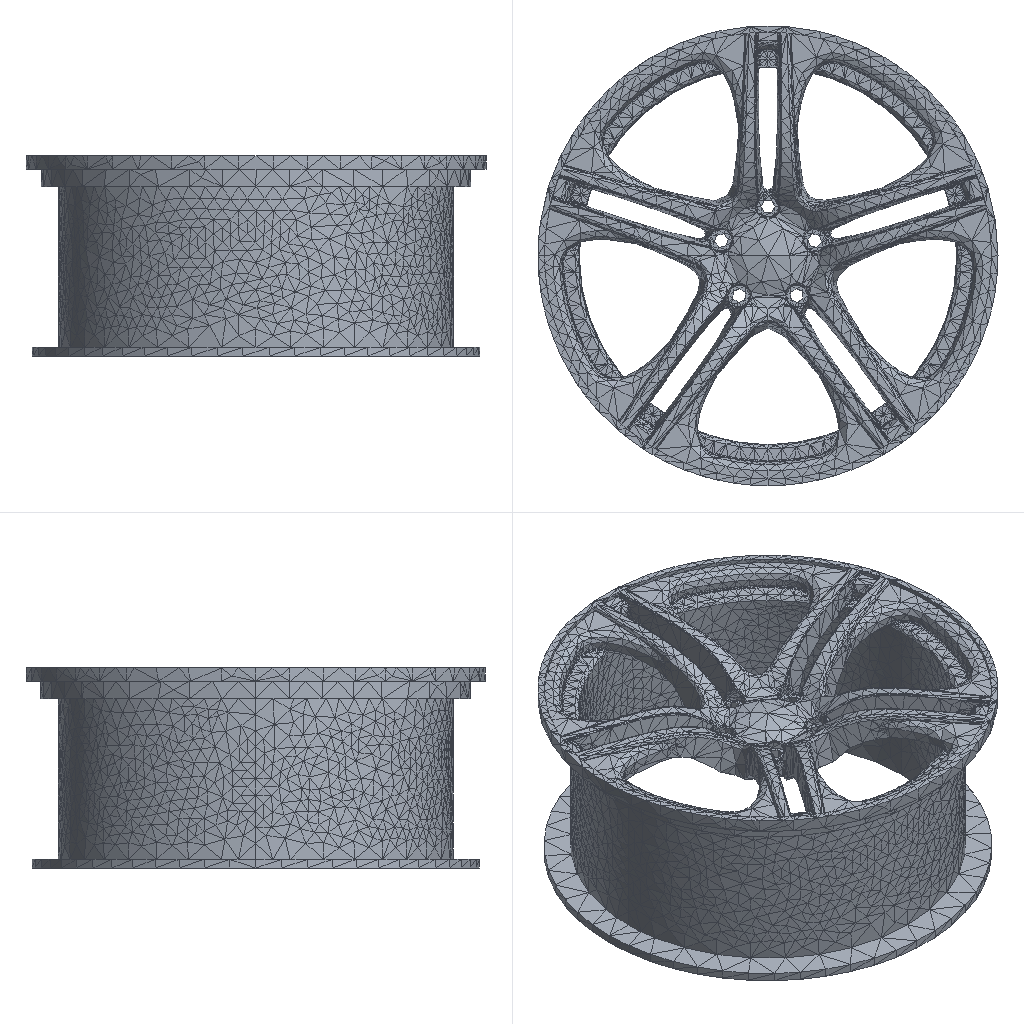Simulation study | ansys workbench
Set-up summary:
category,name,step,type,value,unit,region
solver,ansys_workbench
units,mm-N-s-tonne (MPa),,stated,"/units,MPA"
analysis,LS1,,static
load_step,LS1,LS1,static,nsubst=1; time=1
mesh,nodes,,,48207
mesh,elements,,,28205
element_type,SOLID187,,,25767
element_type,SURF154,,,2438
material,Structural Steel,,E,200000,tonne s^-2 mm^-1
material,Structural Steel,,nu,0.3
material,Structural Steel,,density,7.85e-09,tonne mm^-3
material,Structural Steel,,conductivity,60.5,tonne mm s^-3 C^-1
material,Structural Steel,,specific_heat,4.34e+08,mm^2 s^-2 C^-1
material,Structural Steel,,cte,1.2e-05,C^-1
material,Structural Steel,,permeability,10000
material,Structural Steel,,resistivity,0.00017,ohm mm
load,Define Force Using Surface Effect Elements,LS1,surface-effect pres face 2,-0.01932,,SURF154 #2
bc,Fixed Supports,model,fixed,[dofs=ALL],,_FIXEDSU
named_set,______,,node,549
named_set,_FIXEDSU,,node,549
Ansys APDL input file, long lists of numbers shortened:
/batch
/config,noeldb,1     ! force off writing results to database
*get,_wallstrt,active,,time,wall
! ANSYS input file written by Workbench version 2022 R1
! File used for geometry attach:
/title,wbnew--____ (B5)
! ****** Begin Custom Load Command Snippet ******
/COM, ACT Extensions:
/COM,     LSDYNA, 2021.1
/COM,
! ****** End   Custom Load Command Snippet ******
*DIM,_wb_ProjectScratch_dir,string,248
_wb_ProjectScratch_dir(1) = ''
*DIM,_wb_SolverFiles_dir,string,248
_wb_SolverFiles_dir(1) = ''
*DIM,_wb_userfiles_dir,string,248
_wb_userfiles_dir(1) = ''
/com,--- Data in consistent NMM units. See Solving Units in the help system for more information.
/units,MPA
/nopr
/wb,file,start              !  signify a WB generated input file
/prep7
! Turn off shape checking because checks already performed inside WB mesher.
! See help system for more information.
SHPP,OFF,,NOWARN
/nolist
etcon,set             ! allow ANSYS to choose best KEYOP's for 180x elements, resets any applicable keyopt to MAPDL defaults
/com,*********** Nodes for the whole assembly ***********
nblock,3,,53027
(1i9,3e20.9e3)
        1     8.307477225E+01    -1.054488018E+01     8.547377848E+01
! (48206 more lines like these left out)
-1
/wb,elem,start            !  set before creation of elements
/com,*********** Elements for Body 1 "____-FreeParts|RIM[1]" ***********
et,1,187
eblock,19,solid,,25767
(19i9)
        1        1        1        1        0        0        0        0       10        0        1     1683     3030     1743     7730    21022    21875    21021    21039
! (51533 more lines like these left out)
-1
/wb,elem,end               !  done creating elements
/com,*********** Send User Defined Coordinate System(s) ***********
csys,0
toffst,273.15,  ! Temperature offset from absolute zero
/com,*********** Set Reference Temperature ***********
tref,22.
/wb,mat,start              !  starting to send materials
/com,*********** Send Materials ***********
Temperature = 'TEMP' ! Temperature
MP,DENS,1,7.85e-09,	! tonne mm^-3
MP,ALPX,1,1.2e-05,	! C^-1
MP,C,1,434000000,	! mm^2 s^-2 C^-1
MP,KXX,1,60.5,	! tonne mm s^-3 C^-1
MP,RSVX,1,0.00017,	! ohm mm
MP,EX,1,200000,	! tonne s^-2 mm^-1
MP,NUXY,1,0.3,
MP,MURX,1,10000,
/wb,mat,end                !  done sending materials
!************************* Model Summary ********************
!____-FreeParts|RIM[1],	结构钢,	matid,	1
!************************* End Model Summary ********************
! get the diagonal of the bounding box. Needed later for other things
*get,_xmin,node,,mnloc,x
*get,_ymin,node,,mnloc,y
*get,_zmin,node,,mnloc,z
*get,_xmax,node,,mxloc,x
*get,_ymax,node,,mxloc,y
*get,_zmax,node,,mxloc,z
_ASMDIAG=(_xmax-_xmin)*(_xmax-_xmin)+(_ymax-_ymin)*(_ymax-_ymin)+(_zmax-_zmin)*(_zmax-_zmin)
_ASMDIAG=SQRT(_ASMDIAG)
/wb,contact,start          !  starting to send contact
/wb,contact,end            !  done creating contacts
/com,*********** Send Named Selection as Node Component ***********
CMBLOCK,______  ,NODE,      549
(8i10)
        90        91        92        93       151       152       163       164
! (68 more lines like these left out)
/golist
/wb,load,start             !  starting to send loads
/com,*********** Fixed Supports ***********
CMBLOCK,_FIXEDSU,NODE,      549
(8i10)
        90        91        92        93       151       152       163       164
! (68 more lines like these left out)
cmsel,s,_FIXEDSU
d,all,all
nsel,all
/com,*********** Define Force Using Surface Effect Elements ***********
local,12,0,0.,0.,0.,0.,0.,0.
csys,0
et,2,154
eblock,10,,,2438
(15i9)
    39136        2        2        2       12     1969       74     5447     5447     8846     8850     5447    23519
! (2437 more lines like these left out)
-1
esel,s,type,,2
keyop,2,2,1                ! Apply load in local coordinate system
keyop,2,7,1                ! Use original area so load is constant in large deformation
esel,all
/gst,on,on
fini
*get,_numnode,node,0,count
*get,_numelem,elem,0,count
*get, _MAXELEMNUM, elem, 0, NUM, MAX
*get, _MAXNODENUM, node, 0, NUM, MAX
*get, _MAXELEMTYPE, etyp, 0, NUM, MAX
*get, _MAXREALCONST, real, 0, NUM, MAX
/go
/wb,load,end               !  done creating loads
/com,--- Number of total nodes = %_numnode%
/com,--- Number of contact elements = 2438
/com,--- Number of spring elements = 0
/com,--- Number of bearing elements = 0
/com,--- Number of solid elements = 25767
/com,--- Number of condensed parts = 0
/com,--- Number of total elements = %_numelem%
*get,_wallbsol,active,,time,wall
/com,****************************************************************************
/com,*************************    SOLUTION       ********************************
/com,****************************************************************************
/solu
antype,0                   ! static analysis
_thickRatio=  1     ! Ratio of thick parts in the model
eqsl,pcg,1e-8,,,,,,1
cntr,print,1               ! print out contact info and also make no initial contact an error
dmpoption,emat,no             ! Don't combine emat file for DANSYS
dmpoption,esav,no             ! Don't combine esav file for DANSYS
nldiag,cont,iter           ! print out contact info each equilibrium iteration
rescontrol,,none                 ! Do not keep any restart files
/com,****************************************************
/com,******************* SOLVE FOR LS 1 OF 1 ****************
esel,s,type,,2
nsle
sfe,all,1,pres,1,0.
sfe,all,2,pres,1,-1.93216319958914e-002
sfe,all,3,pres,1,0.
nsel,all
esel,all
/nopr
/gopr
nsub,1,1,1
time,1.
outres,erase
outres,all,none
outres,nsol,all,
outres,rsol,all
outres,eangl,all
outres,etmp,all
outres,veng,all
outres,strs,all,
outres,epel,all,
outres,eppl,all,
outres,cont,all,
! *********** WB SOLVE COMMAND ***********
! check interactive state
*get,ANSINTER_,active,,int
*if,ANSINTER_,ne,0,then
/eof
*endif
solve
/com *************** Write FE CONNECTORS *********
CEWRITE,file,ce,,INTE
/com,****************************************************
/com,*************** FINISHED SOLVE FOR LS 1 *************
*get,_wallasol,active,,time,wall
/nopr
*get,_numnode,node,0,count
*get,_numelem,elem,0,count
*get, _MAXELEMNUM, elem, 0, NUM, MAX
*get, _MAXNODENUM, node, 0, NUM, MAX,,,INTERNAL
*get, _MAXELEMTYPE, etyp, 0, NUM, MAX
*get, _MAXREALCONST, real, 0, NUM, MAX
/gopr
*get,_PCGITER,active,,solu,cgiter
/post1
xmlo,ENCODING,ISO-8859-1
xmlo,parm
/xml,parm,xml
fini
/gopr
*get,_walldone,active,,time,wall
_preptime=(_wallbsol-_wallstrt)*3600
_solvtime=(_wallasol-_wallbsol)*3600
_posttime=(_walldone-_wallasol)*3600
_totaltim=(_walldone-_wallstrt)*3600
*get,_dlbratio,active,0,solu,dlbr
*get,_combtime,active,0,solu,comb
*get,_ssmode,active,0,solu,ssmm
*get,_ndofs,active,0,solu,ndof
*get,_sol_end_time,active,0,set,time
*if,_sol_end_time,eq,1.,then
/fclean				!clean distributed files
*endif
/com,--- Total number of nodes = %_numnode%
/com,--- Total number of elements = %_numelem%
/com,--- Element load balance ratio = %_dlbratio%
/com,--- Time to combine distributed files = %_combtime%
/com,--- Sparse memory mode = %_ssmode%
/com,--- Number of DOF = %_ndofs%
/wb,file,end               ! done with WB generated input
Results summary:
result,analyses[0].index,,,1
result,analyses[0].system,,,SYS
result,analyses[0].deck,,,deck.dat
result,analyses[0].solve_status,,,completed
result,analyses[0].analysis_type,,,static
result,analyses[0].physics,,,mechanical
result,analyses[0].unit_system,,,"NMM: mm, ton, N, s, mV, mA, degC"
result,analyses[0].n_sets,,,1
result,analyses[0].load_steps[0].set,set=1,,1
result,analyses[0].load_steps[0].time_or_freq,set=1,,1
result,analyses[0].load_steps[0].max_displacement_magnitude,set=1,,0.05377
result,analyses[0].load_steps[0].max_von_mises_nodal,set=1,,13.708
result,analyses[0].load_steps[0].reaction_force_sum_xyz[1],set=1,,-3.59664e-06
result,analyses[0].load_steps[0].reaction_force_sum_xyz[2],set=1,,5000
result,analyses[0].load_steps[0].reaction_force_sum_xyz[3],set=1,,6.30575e-06